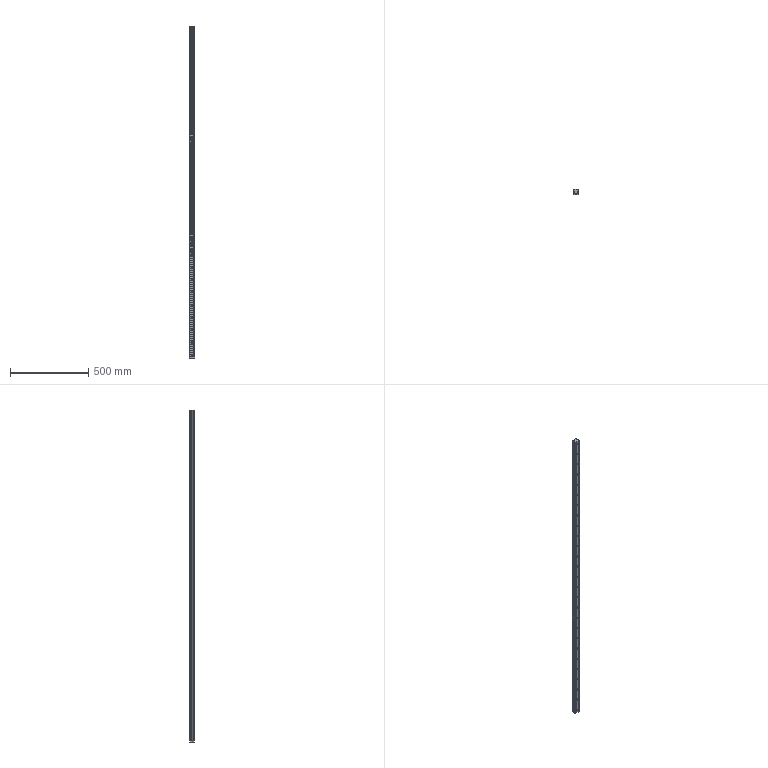Part | STEP file | Linear rail HG35  L2120 (HIWIN) | 1 solid | 283 faces | box 34 x 29 x 2120 mm | volume 1725609 mm3 | plane 134 | cylinder 118 | spline 31 | commonest cylinder face diameters 9 x54 14 x44 15 x10 2.4 x6 6.5 x4